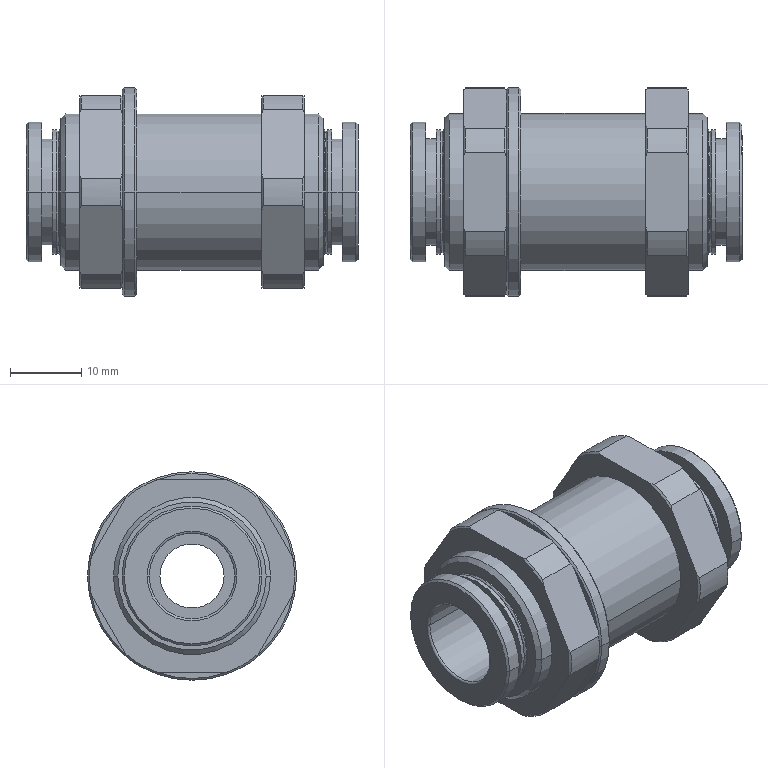Part | SolidWorks | features BaseBody 1 | 1 solid | 128 faces | box 46.5 x 29.2 x 29.2 mm | volume 14559 mm3 | cone 48 | cylinder 44 | plane 32 | torus 4 | commonest cylinder face diameters 29.2 x16 17.5 x8 22 x6 12 x4 14.9 x4 19.6 x4